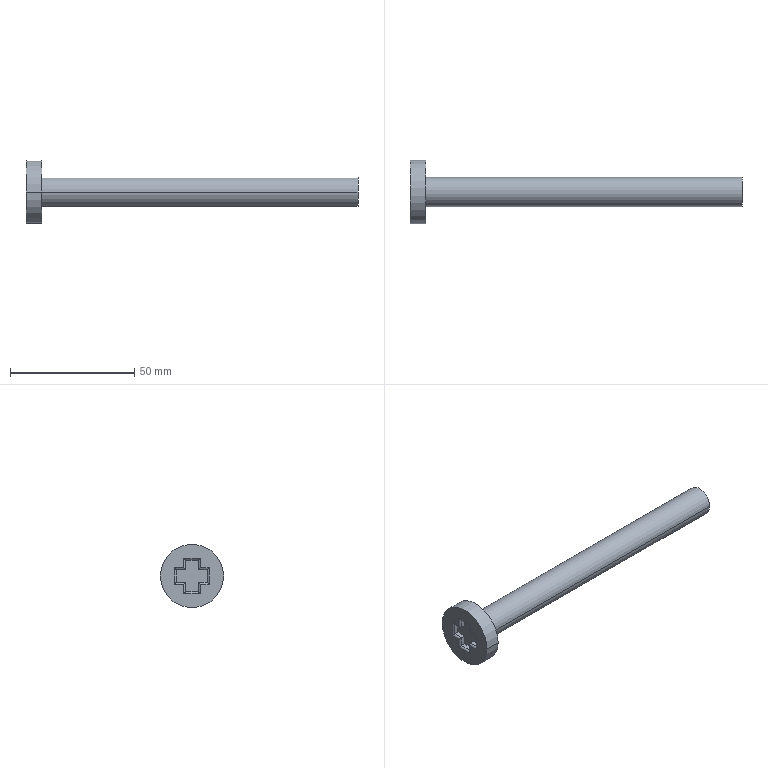Part | SolidWorks | features Fillet 1, ICE 1, Revolution 1 | 1 solid | 32 faces | box 133.35 x 25.4 x 25.4 mm | volume 16568 mm3 | cylinder 16 | plane 16 | commonest cylinder face diameters 1.626 x12 11.684 x2 25.4 x2
STEP:
#1=CARTESIAN_POINT('',(-0.25,0.5,0.));
#2=VERTEX_POINT('',#1);
#3=CARTESIAN_POINT('',(-0.25,-0.5,0.));
#4=VERTEX_POINT('',#3);
#5=CARTESIAN_POINT('',(-0.25,0.,0.));
#6=DIRECTION('',(1.,0.,0.));
#7=DIRECTION('',(0.,1.,0.));
#8=AXIS2_PLACEMENT_3D('',#5,#6,#7);
#9=CIRCLE('',#8,0.5);
#10=EDGE_CURVE('',#2,#4,#9,.T.);
#11=ORIENTED_EDGE('',*,*,#10,.T.);
#12=CARTESIAN_POINT('',(0.,-0.5,0.));
#13=VERTEX_POINT('',#12);
#14=CARTESIAN_POINT('',(5.,-0.5,0.));
#15=DIRECTION('',(1.,0.,0.));
#16=VECTOR('',#15,39.37);
#17=LINE('',#14,#16);
#18=EDGE_CURVE('',#4,#13,#17,.T.);
#19=ORIENTED_EDGE('',*,*,#18,.T.);
#20=CARTESIAN_POINT('',(0.,0.5,0.));
#21=VERTEX_POINT('',#20);
#22=CARTESIAN_POINT('',(0.,0.,0.));
#23=DIRECTION('',(1.,0.,0.));
#24=DIRECTION('',(0.,1.,0.));
#25=AXIS2_PLACEMENT_3D('',#22,#23,#24);
#26=CIRCLE('',#25,0.5);
#27=EDGE_CURVE('',#21,#13,#26,.T.);
#28=ORIENTED_EDGE('',*,*,#27,.F.);
#29=CARTESIAN_POINT('',(5.,0.5,0.));
#30=DIRECTION('',(1.,0.,0.));
#31=VECTOR('',#30,39.37);
#32=LINE('',#29,#31);
#33=EDGE_CURVE('',#2,#21,#32,.T.);
#34=ORIENTED_EDGE('',*,*,#33,.F.);
#35=EDGE_LOOP('',(#11,#19,#28,#34));
#36=FACE_OUTER_BOUND('',#35,.T.);
#37=CARTESIAN_POINT('',(5.,0.,0.));
#38=DIRECTION('',(1.,0.,0.));
#39=DIRECTION('',(0.,1.,0.));
#40=AXIS2_PLACEMENT_3D('',#37,#38,#39);
#41=CYLINDRICAL_SURFACE('',#40,0.5);
#42=ADVANCED_FACE('',(#36),#41,.T.);
#43=CARTESIAN_POINT('',(0.,0.23,0.));
#44=VERTEX_POINT('',#43);
#45=CARTESIAN_POINT('',(0.,-0.23,0.));
#46=VERTEX_POINT('',#45);
#47=CARTESIAN_POINT('',(0.,0.,0.));
#48=DIRECTION('',(1.,0.,0.));
#49=DIRECTION('',(0.,1.,0.));
#50=AXIS2_PLACEMENT_3D('',#47,#48,#49);
#51=CIRCLE('',#50,0.23);
#52=EDGE_CURVE('',#44,#46,#51,.T.);
#53=ORIENTED_EDGE('',*,*,#52,.T.);
#54=CARTESIAN_POINT('',(5.,-0.23,0.));
#55=VERTEX_POINT('',#54);
#56=CARTESIAN_POINT('',(5.,-0.23,0.));
#57=DIRECTION('',(1.,0.,0.));
#58=VECTOR('',#57,39.37);
#59=LINE('',#56,#58);
#60=EDGE_CURVE('',#46,#55,#59,.T.);
#61=ORIENTED_EDGE('',*,*,#60,.T.);
#62=CARTESIAN_POINT('',(5.,0.23,0.));
#63=VERTEX_POINT('',#62);
#64=CARTESIAN_POINT('',(5.,0.,0.));
#65=DIRECTION('',(1.,0.,0.));
#66=DIRECTION('',(0.,1.,0.));
#67=AXIS2_PLACEMENT_3D('',#64,#65,#66);
#68=CIRCLE('',#67,0.23);
#69=EDGE_CURVE('',#63,#55,#68,.T.);
#70=ORIENTED_EDGE('',*,*,#69,.F.);
#71=CARTESIAN_POINT('',(5.,0.23,0.));
#72=DIRECTION('',(1.,0.,0.));
#73=VECTOR('',#72,39.37);
#74=LINE('',#71,#73);
#75=EDGE_CURVE('',#44,#63,#74,.T.);
#76=ORIENTED_EDGE('',*,*,#75,.F.);
#77=EDGE_LOOP('',(#53,#61,#70,#76));
#78=FACE_OUTER_BOUND('',#77,.T.);
#79=CARTESIAN_POINT('',(5.,0.,0.));
#80=DIRECTION('',(1.,0.,0.));
#81=DIRECTION('',(0.,1.,0.));
#82=AXIS2_PLACEMENT_3D('',#79,#80,#81);
#83=CYLINDRICAL_SURFACE('',#82,0.23);
#84=ADVANCED_FACE('',(#78),#83,.T.);
#85=ORIENTED_EDGE('',*,*,#69,.T.);
#86=CARTESIAN_POINT('',(5.,0.,0.));
#87=DIRECTION('',(1.,0.,0.));
#88=DIRECTION('',(0.,1.,0.));
#89=AXIS2_PLACEMENT_3D('',#86,#87,#88);
#90=CIRCLE('',#89,0.23);
#91=EDGE_CURVE('',#55,#63,#90,.T.);
#92=ORIENTED_EDGE('',*,*,#91,.T.);
#93=EDGE_LOOP('',(#85,#92));
#94=FACE_OUTER_BOUND('',#93,.T.);
#95=CARTESIAN_POINT('',(5.,0.23,0.));
#96=DIRECTION('',(1.,0.,0.));
#97=DIRECTION('',(0.,1.,0.));
#98=AXIS2_PLACEMENT_3D('',#95,#96,#97);
#99=PLANE('',#98);
#100=ADVANCED_FACE('',(#94),#99,.T.);
#101=ORIENTED_EDGE('',*,*,#60,.F.);
#102=CARTESIAN_POINT('',(0.,0.,0.));
#103=DIRECTION('',(1.,0.,0.));
#104=DIRECTION('',(0.,1.,0.));
#105=AXIS2_PLACEMENT_3D('',#102,#103,#104);
#106=CIRCLE('',#105,0.23);
#107=EDGE_CURVE('',#46,#44,#106,.T.);
#108=ORIENTED_EDGE('',*,*,#107,.T.);
#109=ORIENTED_EDGE('',*,*,#75,.T.);
#110=ORIENTED_EDGE('',*,*,#91,.F.);
#111=EDGE_LOOP('',(#101,#108,#109,#110));
#112=FACE_OUTER_BOUND('',#111,.T.);
#113=CARTESIAN_POINT('',(5.,0.,0.));
#114=DIRECTION('',(1.,0.,0.));
#115=DIRECTION('',(0.,1.,0.));
#116=AXIS2_PLACEMENT_3D('',#113,#114,#115);
#117=CYLINDRICAL_SURFACE('',#116,0.23);
#118=ADVANCED_FACE('',(#112),#117,.T.);
#119=ORIENTED_EDGE('',*,*,#27,.T.);
#120=CARTESIAN_POINT('',(0.,0.,0.));
#121=DIRECTION('',(1.,0.,0.));
#122=DIRECTION('',(0.,1.,0.));
#123=AXIS2_PLACEMENT_3D('',#120,#121,#122);
#124=CIRCLE('',#123,0.5);
#125=EDGE_CURVE('',#13,#21,#124,.T.);
#126=ORIENTED_EDGE('',*,*,#125,.T.);
#127=EDGE_LOOP('',(#119,#126));
#128=FACE_OUTER_BOUND('',#127,.T.);
#129=ORIENTED_EDGE('',*,*,#52,.F.);
#130=ORIENTED_EDGE('',*,*,#107,.F.);
#131=EDGE_LOOP('',(#129,#130));
#132=FACE_BOUND('',#131,.T.);
#133=CARTESIAN_POINT('',(0.,0.23,0.));
#134=DIRECTION('',(1.,0.,0.));
#135=DIRECTION('',(0.,1.,0.));
#136=AXIS2_PLACEMENT_3D('',#133,#134,#135);
#137=PLANE('',#136);
#138=ADVANCED_FACE('',(#128,#132),#137,.T.);
#139=ORIENTED_EDGE('',*,*,#18,.F.);
#140=CARTESIAN_POINT('',(-0.25,0.,0.));
#141=DIRECTION('',(1.,0.,0.));
#142=DIRECTION('',(0.,1.,0.));
#143=AXIS2_PLACEMENT_3D('',#140,#141,#142);
#144=CIRCLE('',#143,0.5);
#145=EDGE_CURVE('',#4,#2,#144,.T.);
#146=ORIENTED_EDGE('',*,*,#145,.T.);
#147=ORIENTED_EDGE('',*,*,#33,.T.);
#148=ORIENTED_EDGE('',*,*,#125,.F.);
#149=EDGE_LOOP('',(#139,#146,#147,#148));
#150=FACE_OUTER_BOUND('',#149,.T.);
#151=CARTESIAN_POINT('',(5.,0.,0.));
#152=DIRECTION('',(1.,0.,0.));
#153=DIRECTION('',(0.,1.,0.));
#154=AXIS2_PLACEMENT_3D('',#151,#152,#153);
#155=CYLINDRICAL_SURFACE('',#154,0.5);
#156=ADVANCED_FACE('',(#150),#155,.T.);
#157=CARTESIAN_POINT('',(-0.25,-0.132,0.132));
#158=VERTEX_POINT('',#157);
#159=CARTESIAN_POINT('',(-0.25,-0.273,0.132));
#160=VERTEX_POINT('',#159);
#161=CARTESIAN_POINT('',(-0.25,-0.241,0.132));
#162=DIRECTION('',(0.,-1.,0.));
#163=VECTOR('',#162,39.37);
#164=LINE('',#161,#163);
#165=EDGE_CURVE('',#158,#160,#164,.T.);
#166=ORIENTED_EDGE('',*,*,#165,.T.);
#167=CARTESIAN_POINT('',(-0.25,-0.273,-0.132));
#168=VERTEX_POINT('',#167);
#169=CARTESIAN_POINT('',(-0.25,-0.273,-0.1));
#170=DIRECTION('',(0.,0.,-1.));
#171=VECTOR('',#170,39.37);
#172=LINE('',#169,#171);
#173=EDGE_CURVE('',#160,#168,#172,.T.);
#174=ORIENTED_EDGE('',*,*,#173,.T.);
#175=CARTESIAN_POINT('',(-0.25,-0.132,-0.132));
#176=VERTEX_POINT('',#175);
#177=CARTESIAN_POINT('',(-0.25,-0.1,-0.132));
#178=DIRECTION('',(0.,1.,0.));
#179=VECTOR('',#178,39.37);
#180=LINE('',#177,#179);
#181=EDGE_CURVE('',#168,#176,#180,.T.);
#182=ORIENTED_EDGE('',*,*,#181,.T.);
#183=CARTESIAN_POINT('',(-0.25,-0.132,-0.282));
#184=VERTEX_POINT('',#183);
#185=CARTESIAN_POINT('',(-0.25,-0.132,-0.25));
#186=DIRECTION('',(0.,0.,-1.));
#187=VECTOR('',#186,39.37);
#188=LINE('',#185,#187);
#189=EDGE_CURVE('',#176,#184,#188,.T.);
#190=ORIENTED_EDGE('',*,*,#189,.T.);
#191=CARTESIAN_POINT('',(-0.25,0.132,-0.282));
#192=VERTEX_POINT('',#191);
#193=CARTESIAN_POINT('',(-0.25,0.1,-0.282));
#194=DIRECTION('',(0.,1.,0.));
#195=VECTOR('',#194,39.37);
#196=LINE('',#193,#195);
#197=EDGE_CURVE('',#184,#192,#196,.T.);
#198=ORIENTED_EDGE('',*,*,#197,.T.);
#199=CARTESIAN_POINT('',(-0.25,0.132,-0.132));
#200=VERTEX_POINT('',#199);
#201=CARTESIAN_POINT('',(-0.25,0.132,-0.1));
#202=DIRECTION('',(0.,0.,1.));
#203=VECTOR('',#202,39.37);
#204=LINE('',#201,#203);
#205=EDGE_CURVE('',#192,#200,#204,.T.);
#206=ORIENTED_EDGE('',*,*,#205,.T.);
#207=CARTESIAN_POINT('',(-0.25,0.282,-0.132));
#208=VERTEX_POINT('',#207);
#209=CARTESIAN_POINT('',(-0.25,0.25,-0.132));
#210=DIRECTION('',(0.,1.,0.));
#211=VECTOR('',#210,39.37);
#212=LINE('',#209,#211);
#213=EDGE_CURVE('',#200,#208,#212,.T.);
#214=ORIENTED_EDGE('',*,*,#213,.T.);
#215=CARTESIAN_POINT('',(-0.25,0.282,0.132));
#216=VERTEX_POINT('',#215);
#217=CARTESIAN_POINT('',(-0.25,0.282,0.1));
#218=DIRECTION('',(0.,0.,1.));
#219=VECTOR('',#218,39.37);
#220=LINE('',#217,#219);
#221=EDGE_CURVE('',#208,#216,#220,.T.);
#222=ORIENTED_EDGE('',*,*,#221,.T.);
#223=CARTESIAN_POINT('',(-0.25,0.132,0.132));
#224=VERTEX_POINT('',#223);
#225=CARTESIAN_POINT('',(-0.25,0.1,0.132));
#226=DIRECTION('',(0.,-1.,0.));
#227=VECTOR('',#226,39.37);
#228=LINE('',#225,#227);
#229=EDGE_CURVE('',#216,#224,#228,.T.);
#230=ORIENTED_EDGE('',*,*,#229,.T.);
#231=CARTESIAN_POINT('',(-0.25,0.132,0.282));
#232=VERTEX_POINT('',#231);
#233=CARTESIAN_POINT('',(-0.25,0.132,0.25));
#234=DIRECTION('',(0.,0.,1.));
#235=VECTOR('',#234,39.37);
#236=LINE('',#233,#235);
#237=EDGE_CURVE('',#224,#232,#236,.T.);
#238=ORIENTED_EDGE('',*,*,#237,.T.);
#239=CARTESIAN_POINT('',(-0.25,-0.132,0.282));
#240=VERTEX_POINT('',#239);
#241=CARTESIAN_POINT('',(-0.25,-0.1,0.282));
#242=DIRECTION('',(0.,-1.,0.));
#243=VECTOR('',#242,39.37);
#244=LINE('',#241,#243);
#245=EDGE_CURVE('',#232,#240,#244,.T.);
#246=ORIENTED_EDGE('',*,*,#245,.T.);
#247=CARTESIAN_POINT('',(-0.25,-0.132,0.1));
#248=DIRECTION('',(0.,0.,-1.));
#249=VECTOR('',#248,39.37);
#250=LINE('',#247,#249);
#251=EDGE_CURVE('',#240,#158,#250,.T.);
#252=ORIENTED_EDGE('',*,*,#251,.T.);
#253=EDGE_LOOP('',(#166,#174,#182,#190,#198,#206,#214,#222,#230,#238,#246,#252));
#254=FACE_BOUND('',#253,.T.);
#255=ORIENTED_EDGE('',*,*,#10,.F.);
#256=ORIENTED_EDGE('',*,*,#145,.F.);
#257=EDGE_LOOP('',(#255,#256));
#258=FACE_OUTER_BOUND('',#257,.T.);
#259=CARTESIAN_POINT('',(-0.25,0.5,0.));
#260=DIRECTION('',(-1.,0.,0.));
#261=DIRECTION('',(0.,-1.,0.));
#262=AXIS2_PLACEMENT_3D('',#259,#260,#261);
#263=PLANE('',#262);
#264=ADVANCED_FACE('',(#254,#258),#263,.T.);
#265=CARTESIAN_POINT('',(-0.15,0.25,0.1));
#266=VERTEX_POINT('',#265);
#267=CARTESIAN_POINT('',(-0.218,0.25,0.1));
#268=VERTEX_POINT('',#267);
#269=CARTESIAN_POINT('',(-0.15,0.25,0.1));
#270=DIRECTION('',(-1.,0.,0.));
#271=VECTOR('',#270,39.37);
#272=LINE('',#269,#271);
#273=EDGE_CURVE('',#266,#268,#272,.T.);
#274=ORIENTED_EDGE('',*,*,#273,.T.);
#275=CARTESIAN_POINT('',(-0.218,0.25,-0.1));
#276=VERTEX_POINT('',#275);
#277=CARTESIAN_POINT('',(-0.218,0.25,-0.1));
#278=DIRECTION('',(0.,0.,-1.));
#279=VECTOR('',#278,39.37);
#280=LINE('',#277,#279);
#281=EDGE_CURVE('',#268,#276,#280,.T.);
#282=ORIENTED_EDGE('',*,*,#281,.T.);
#283=CARTESIAN_POINT('',(-0.15,0.25,-0.1));
#284=VERTEX_POINT('',#283);
#285=CARTESIAN_POINT('',(-0.15,0.25,-0.1));
#286=DIRECTION('',(-1.,0.,0.));
#287=VECTOR('',#286,39.37);
#288=LINE('',#285,#287);
#289=EDGE_CURVE('',#284,#276,#288,.T.);
#290=ORIENTED_EDGE('',*,*,#289,.F.);
#291=CARTESIAN_POINT('',(-0.15,0.25,-0.1));
#292=DIRECTION('',(0.,0.,-1.));
#293=VECTOR('',#292,39.37);
#294=LINE('',#291,#293);
#295=EDGE_CURVE('',#266,#284,#294,.T.);
#296=ORIENTED_EDGE('',*,*,#295,.F.);
#297=EDGE_LOOP('',(#274,#282,#290,#296));
#298=FACE_OUTER_BOUND('',#297,.T.);
#299=CARTESIAN_POINT('',(-0.15,0.25,-0.1));
#300=DIRECTION('',(0.,1.,0.));
#301=DIRECTION('',(-1.,0.,0.));
#302=AXIS2_PLACEMENT_3D('',#299,#300,#301);
#303=PLANE('',#302);
#304=ADVANCED_FACE('',(#298),#303,.F.);
#305=CARTESIAN_POINT('',(-0.15,0.1,0.1));
#306=VERTEX_POINT('',#305);
#307=CARTESIAN_POINT('',(-0.218,0.1,0.1));
#308=VERTEX_POINT('',#307);
#309=CARTESIAN_POINT('',(-0.15,0.1,0.1));
#310=DIRECTION('',(-1.,0.,0.));
#311=VECTOR('',#310,39.37);
#312=LINE('',#309,#311);
#313=EDGE_CURVE('',#306,#308,#312,.T.);
#314=ORIENTED_EDGE('',*,*,#313,.T.);
#315=CARTESIAN_POINT('',(-0.218,0.25,0.1));
#316=DIRECTION('',(0.,1.,0.));
#317=VECTOR('',#316,39.37);
#318=LINE('',#315,#317);
#319=EDGE_CURVE('',#308,#268,#318,.T.);
#320=ORIENTED_EDGE('',*,*,#319,.T.);
#321=ORIENTED_EDGE('',*,*,#273,.F.);
#322=CARTESIAN_POINT('',(-0.15,0.25,0.1));
#323=DIRECTION('',(0.,1.,0.));
#324=VECTOR('',#323,39.37);
#325=LINE('',#322,#324);
#326=EDGE_CURVE('',#306,#266,#325,.T.);
#327=ORIENTED_EDGE('',*,*,#326,.F.);
#328=EDGE_LOOP('',(#314,#320,#321,#327));
#329=FACE_OUTER_BOUND('',#328,.T.);
#330=CARTESIAN_POINT('',(-0.15,0.25,0.1));
#331=DIRECTION('',(0.,0.,1.));
#332=DIRECTION('',(0.,-1.,0.));
#333=AXIS2_PLACEMENT_3D('',#330,#331,#332);
#334=PLANE('',#333);
#335=ADVANCED_FACE('',(#329),#334,.F.);
#336=CARTESIAN_POINT('',(-0.15,0.1,0.25));
#337=VERTEX_POINT('',#336);
#338=CARTESIAN_POINT('',(-0.218,0.1,0.25));
#339=VERTEX_POINT('',#338);
#340=CARTESIAN_POINT('',(-0.15,0.1,0.25));
#341=DIRECTION('',(-1.,0.,0.));
#342=VECTOR('',#341,39.37);
#343=LINE('',#340,#342);
#344=EDGE_CURVE('',#337,#339,#343,.T.);
#345=ORIENTED_EDGE('',*,*,#344,.T.);
#346=CARTESIAN_POINT('',(-0.218,0.1,0.1));
#347=DIRECTION('',(0.,0.,-1.));
#348=VECTOR('',#347,39.37);
#349=LINE('',#346,#348);
#350=EDGE_CURVE('',#339,#308,#349,.T.);
#351=ORIENTED_EDGE('',*,*,#350,.T.);
#352=ORIENTED_EDGE('',*,*,#313,.F.);
#353=CARTESIAN_POINT('',(-0.15,0.1,0.1));
#354=DIRECTION('',(0.,0.,-1.));
#355=VECTOR('',#354,39.37);
#356=LINE('',#353,#355);
#357=EDGE_CURVE('',#337,#306,#356,.T.);
#358=ORIENTED_EDGE('',*,*,#357,.F.);
#359=EDGE_LOOP('',(#345,#351,#352,#358));
#360=FACE_OUTER_BOUND('',#359,.T.);
#361=CARTESIAN_POINT('',(-0.15,0.1,0.1));
#362=DIRECTION('',(0.,1.,0.));
#363=DIRECTION('',(-1.,0.,0.));
#364=AXIS2_PLACEMENT_3D('',#361,#362,#363);
#365=PLANE('',#364);
#366=ADVANCED_FACE('',(#360),#365,.F.);
#367=CARTESIAN_POINT('',(-0.15,-0.1,0.25));
#368=VERTEX_POINT('',#367);
#369=CARTESIAN_POINT('',(-0.218,-0.1,0.25));
#370=VERTEX_POINT('',#369);
#371=CARTESIAN_POINT('',(-0.15,-0.1,0.25));
#372=DIRECTION('',(-1.,0.,0.));
#373=VECTOR('',#372,39.37);
#374=LINE('',#371,#373);
#375=EDGE_CURVE('',#368,#370,#374,.T.);
#376=ORIENTED_EDGE('',*,*,#375,.T.);
#377=CARTESIAN_POINT('',(-0.218,0.1,0.25));
#378=DIRECTION('',(0.,1.,0.));
#379=VECTOR('',#378,39.37);
#380=LINE('',#377,#379);
#381=EDGE_CURVE('',#370,#339,#380,.T.);
#382=ORIENTED_EDGE('',*,*,#381,.T.);
#383=ORIENTED_EDGE('',*,*,#344,.F.);
#384=CARTESIAN_POINT('',(-0.15,0.1,0.25));
#385=DIRECTION('',(0.,1.,0.));
#386=VECTOR('',#385,39.37);
#387=LINE('',#384,#386);
#388=EDGE_CURVE('',#368,#337,#387,.T.);
#389=ORIENTED_EDGE('',*,*,#388,.F.);
#390=EDGE_LOOP('',(#376,#382,#383,#389));
#391=FACE_OUTER_BOUND('',#390,.T.);
#392=CARTESIAN_POINT('',(-0.15,0.1,0.25));
#393=DIRECTION('',(0.,0.,1.));
#394=DIRECTION('',(0.,-1.,0.));
#395=AXIS2_PLACEMENT_3D('',#392,#393,#394);
#396=PLANE('',#395);
#397=ADVANCED_FACE('',(#391),#396,.F.);
#398=CARTESIAN_POINT('',(-0.15,-0.1,0.1));
#399=VERTEX_POINT('',#398);
#400=CARTESIAN_POINT('',(-0.218,-0.1,0.1));
#401=VERTEX_POINT('',#400);
#402=CARTESIAN_POINT('',(-0.15,-0.1,0.1));
#403=DIRECTION('',(-1.,0.,0.));
#404=VECTOR('',#403,39.37);
#405=LINE('',#402,#404);
#406=EDGE_CURVE('',#399,#401,#405,.T.);
#407=ORIENTED_EDGE('',*,*,#406,.T.);
#408=CARTESIAN_POINT('',(-0.218,-0.1,0.25));
#409=DIRECTION('',(0.,0.,1.));
#410=VECTOR('',#409,39.37);
#411=LINE('',#408,#410);
#412=EDGE_CURVE('',#401,#370,#411,.T.);
#413=ORIENTED_EDGE('',*,*,#412,.T.);
#414=ORIENTED_EDGE('',*,*,#375,.F.);
#415=CARTESIAN_POINT('',(-0.15,-0.1,0.25));
#416=DIRECTION('',(0.,0.,1.));
#417=VECTOR('',#416,39.37);
#418=LINE('',#415,#417);
#419=EDGE_CURVE('',#399,#368,#418,.T.);
#420=ORIENTED_EDGE('',*,*,#419,.F.);
#421=EDGE_LOOP('',(#407,#413,#414,#420));
#422=FACE_OUTER_BOUND('',#421,.T.);
#423=CARTESIAN_POINT('',(-0.15,-0.1,0.25));
#424=DIRECTION('',(0.,-1.,0.));
#425=DIRECTION('',(0.,0.,-1.));
#426=AXIS2_PLACEMENT_3D('',#423,#424,#425);
#427=PLANE('',#426);
#428=ADVANCED_FACE('',(#422),#427,.F.);
#429=CARTESIAN_POINT('',(-0.15,-0.241,0.1));
#430=VERTEX_POINT('',#429);
#431=CARTESIAN_POINT('',(-0.218,-0.241,0.1));
#432=VERTEX_POINT('',#431);
#433=CARTESIAN_POINT('',(-0.15,-0.241,0.1));
#434=DIRECTION('',(-1.,0.,0.));
#435=VECTOR('',#434,39.37);
#436=LINE('',#433,#435);
#437=EDGE_CURVE('',#430,#432,#436,.T.);
#438=ORIENTED_EDGE('',*,*,#437,.T.);
#439=CARTESIAN_POINT('',(-0.218,-0.1,0.1));
#440=DIRECTION('',(0.,1.,0.));
#441=VECTOR('',#440,39.37);
#442=LINE('',#439,#441);
#443=EDGE_CURVE('',#432,#401,#442,.T.);
#444=ORIENTED_EDGE('',*,*,#443,.T.);
#445=ORIENTED_EDGE('',*,*,#406,.F.);
#446=CARTESIAN_POINT('',(-0.15,-0.1,0.1));
#447=DIRECTION('',(0.,1.,0.));
#448=VECTOR('',#447,39.37);
#449=LINE('',#446,#448);
#450=EDGE_CURVE('',#430,#399,#449,.T.);
#451=ORIENTED_EDGE('',*,*,#450,.F.);
#452=EDGE_LOOP('',(#438,#444,#445,#451));
#453=FACE_OUTER_BOUND('',#452,.T.);
#454=CARTESIAN_POINT('',(-0.15,-0.1,0.1));
#455=DIRECTION('',(0.,0.,1.));
#456=DIRECTION('',(0.,-1.,0.));
#457=AXIS2_PLACEMENT_3D('',#454,#455,#456);
#458=PLANE('',#457);
#459=ADVANCED_FACE('',(#453),#458,.F.);
#460=CARTESIAN_POINT('',(-0.15,-0.241,-0.1));
#461=VERTEX_POINT('',#460);
#462=CARTESIAN_POINT('',(-0.218,-0.241,-0.1));
#463=VERTEX_POINT('',#462);
#464=CARTESIAN_POINT('',(-0.15,-0.241,-0.1));
#465=DIRECTION('',(-1.,0.,0.));
#466=VECTOR('',#465,39.37);
#467=LINE('',#464,#466);
#468=EDGE_CURVE('',#461,#463,#467,.T.);
#469=ORIENTED_EDGE('',*,*,#468,.T.);
#470=CARTESIAN_POINT('',(-0.218,-0.241,0.1));
#471=DIRECTION('',(0.,0.,1.));
#472=VECTOR('',#471,39.37);
#473=LINE('',#470,#472);
#474=EDGE_CURVE('',#463,#432,#473,.T.);
#475=ORIENTED_EDGE('',*,*,#474,.T.);
#476=ORIENTED_EDGE('',*,*,#437,.F.);
#477=CARTESIAN_POINT('',(-0.15,-0.241,-0.1));
#478=DIRECTION('',(0.,0.,1.));
#479=VECTOR('',#478,39.37);
#480=LINE('',#477,#479);
#481=EDGE_CURVE('',#461,#430,#480,.T.);
#482=ORIENTED_EDGE('',*,*,#481,.F.);
#483=EDGE_LOOP('',(#469,#475,#476,#482));
#484=FACE_OUTER_BOUND('',#483,.T.);
#485=CARTESIAN_POINT('',(-0.15,-0.241,-0.1));
#486=DIRECTION('',(0.,-1.,0.));
#487=DIRECTION('',(1.,0.,0.));
#488=AXIS2_PLACEMENT_3D('',#485,#486,#487);
#489=PLANE('',#488);
#490=ADVANCED_FACE('',(#484),#489,.F.);
#491=CARTESIAN_POINT('',(-0.15,-0.1,-0.1));
#492=VERTEX_POINT('',#491);
#493=CARTESIAN_POINT('',(-0.218,-0.1,-0.1));
#494=VERTEX_POINT('',#493);
#495=CARTESIAN_POINT('',(-0.15,-0.1,-0.1));
#496=DIRECTION('',(-1.,0.,0.));
#497=VECTOR('',#496,39.37);
#498=LINE('',#495,#497);
#499=EDGE_CURVE('',#492,#494,#498,.T.);
#500=ORIENTED_EDGE('',*,*,#499,.T.);
#501=CARTESIAN_POINT('',(-0.218,-0.241,-0.1));
#502=DIRECTION('',(0.,-1.,0.));
#503=VECTOR('',#502,39.37);
#504=LINE('',#501,#503);
#505=EDGE_CURVE('',#494,#463,#504,.T.);
#506=ORIENTED_EDGE('',*,*,#505,.T.);
#507=ORIENTED_EDGE('',*,*,#468,.F.);
#508=CARTESIAN_POINT('',(-0.15,-0.1,-0.1));
#509=DIRECTION('',(0.,-1.,0.));
#510=VECTOR('',#509,39.37);
#511=LINE('',#508,#510);
#512=EDGE_CURVE('',#492,#461,#511,.T.);
#513=ORIENTED_EDGE('',*,*,#512,.F.);
#514=EDGE_LOOP('',(#500,#506,#507,#513));
#515=FACE_OUTER_BOUND('',#514,.T.);
#516=CARTESIAN_POINT('',(-0.15,-0.1,-0.1));
#517=DIRECTION('',(0.,0.,-1.));
#518=DIRECTION('',(0.,1.,0.));
#519=AXIS2_PLACEMENT_3D('',#516,#517,#518);
#520=PLANE('',#519);
#521=ADVANCED_FACE('',(#515),#520,.F.);
#522=CARTESIAN_POINT('',(-0.15,-0.1,-0.25));
#523=VERTEX_POINT('',#522);
#524=CARTESIAN_POINT('',(-0.218,-0.1,-0.25));
#525=VERTEX_POINT('',#524);
#526=CARTESIAN_POINT('',(-0.15,-0.1,-0.25));
#527=DIRECTION('',(-1.,0.,0.));
#528=VECTOR('',#527,39.37);
#529=LINE('',#526,#528);
#530=EDGE_CURVE('',#523,#525,#529,.T.);
#531=ORIENTED_EDGE('',*,*,#530,.T.);
#532=CARTESIAN_POINT('',(-0.218,-0.1,-0.1));
#533=DIRECTION('',(0.,0.,1.));
#534=VECTOR('',#533,39.37);
#535=LINE('',#532,#534);
#536=EDGE_CURVE('',#525,#494,#535,.T.);
#537=ORIENTED_EDGE('',*,*,#536,.T.);
#538=ORIENTED_EDGE('',*,*,#499,.F.);
#539=CARTESIAN_POINT('',(-0.15,-0.1,-0.25));
#540=DIRECTION('',(0.,0.,1.));
#541=VECTOR('',#540,39.37);
#542=LINE('',#539,#541);
#543=EDGE_CURVE('',#523,#492,#542,.T.);
#544=ORIENTED_EDGE('',*,*,#543,.F.);
#545=EDGE_LOOP('',(#531,#537,#538,#544));
#546=FACE_OUTER_BOUND('',#545,.T.);
#547=CARTESIAN_POINT('',(-0.15,-0.1,-0.25));
#548=DIRECTION('',(0.,-1.,0.));
#549=DIRECTION('',(0.,0.,-1.));
#550=AXIS2_PLACEMENT_3D('',#547,#548,#549);
#551=PLANE('',#550);
#552=ADVANCED_FACE('',(#546),#551,.F.);
#553=CARTESIAN_POINT('',(-0.15,0.1,-0.25));
#554=VERTEX_POINT('',#553);
#555=CARTESIAN_POINT('',(-0.218,0.1,-0.25));
#556=VERTEX_POINT('',#555);
#557=CARTESIAN_POINT('',(-0.15,0.1,-0.25));
#558=DIRECTION('',(-1.,0.,0.));
#559=VECTOR('',#558,39.37);
#560=LINE('',#557,#559);
#561=EDGE_CURVE('',#554,#556,#560,.T.);
#562=ORIENTED_EDGE('',*,*,#561,.T.);
#563=CARTESIAN_POINT('',(-0.218,-0.1,-0.25));
#564=DIRECTION('',(0.,-1.,0.));
#565=VECTOR('',#564,39.37);
#566=LINE('',#563,#565);
#567=EDGE_CURVE('',#556,#525,#566,.T.);
#568=ORIENTED_EDGE('',*,*,#567,.T.);
#569=ORIENTED_EDGE('',*,*,#530,.F.);
#570=CARTESIAN_POINT('',(-0.15,0.1,-0.25));
#571=DIRECTION('',(0.,-1.,0.));
#572=VECTOR('',#571,39.37);
#573=LINE('',#570,#572);
#574=EDGE_CURVE('',#554,#523,#573,.T.);
#575=ORIENTED_EDGE('',*,*,#574,.F.);
#576=EDGE_LOOP('',(#562,#568,#569,#575));
#577=FACE_OUTER_BOUND('',#576,.T.);
#578=CARTESIAN_POINT('',(-0.15,0.1,-0.25));
#579=DIRECTION('',(0.,0.,-1.));
#580=DIRECTION('',(0.,1.,0.));
#581=AXIS2_PLACEMENT_3D('',#578,#579,#580);
#582=PLANE('',#581);
#583=ADVANCED_FACE('',(#577),#582,.F.);
#584=CARTESIAN_POINT('',(-0.15,0.1,-0.1));
#585=VERTEX_POINT('',#584);
#586=CARTESIAN_POINT('',(-0.218,0.1,-0.1));
#587=VERTEX_POINT('',#586);
#588=CARTESIAN_POINT('',(-0.15,0.1,-0.1));
#589=DIRECTION('',(-1.,0.,0.));
#590=VECTOR('',#589,39.37);
#591=LINE('',#588,#590);
#592=EDGE_CURVE('',#585,#587,#591,.T.);
#593=ORIENTED_EDGE('',*,*,#592,.T.);
#594=CARTESIAN_POINT('',(-0.218,0.1,-0.25));
#595=DIRECTION('',(0.,0.,-1.));
#596=VECTOR('',#595,39.37);
#597=LINE('',#594,#596);
#598=EDGE_CURVE('',#587,#556,#597,.T.);
#599=ORIENTED_EDGE('',*,*,#598,.T.);
#600=ORIENTED_EDGE('',*,*,#561,.F.);
#601=CARTESIAN_POINT('',(-0.15,0.1,-0.1));
#602=DIRECTION('',(0.,0.,-1.));
#603=VECTOR('',#602,39.37);
#604=LINE('',#601,#603);
#605=EDGE_CURVE('',#585,#554,#604,.T.);
#606=ORIENTED_EDGE('',*,*,#605,.F.);
#607=EDGE_LOOP('',(#593,#599,#600,#606));
#608=FACE_OUTER_BOUND('',#607,.T.);
#609=CARTESIAN_POINT('',(-0.15,0.1,-0.1));
#610=DIRECTION('',(0.,1.,0.));
#611=DIRECTION('',(-1.,0.,0.));
#612=AXIS2_PLACEMENT_3D('',#609,#610,#611);
#613=PLANE('',#612);
#614=ADVANCED_FACE('',(#608),#613,.F.);
#615=ORIENTED_EDGE('',*,*,#289,.T.);
#616=CARTESIAN_POINT('',(-0.218,0.1,-0.1));
#617=DIRECTION('',(0.,-1.,0.));
#618=VECTOR('',#617,39.37);
#619=LINE('',#616,#618);
#620=EDGE_CURVE('',#276,#587,#619,.T.);
#621=ORIENTED_EDGE('',*,*,#620,.T.);
#622=ORIENTED_EDGE('',*,*,#592,.F.);
#623=CARTESIAN_POINT('',(-0.15,0.25,-0.1));
#624=DIRECTION('',(0.,-1.,0.));
#625=VECTOR('',#624,39.37);
#626=LINE('',#623,#625);
#627=EDGE_CURVE('',#284,#585,#626,.T.);
#628=ORIENTED_EDGE('',*,*,#627,.F.);
#629=EDGE_LOOP('',(#615,#621,#622,#628));
#630=FACE_OUTER_BOUND('',#629,.T.);
#631=CARTESIAN_POINT('',(-0.15,0.25,-0.1));
#632=DIRECTION('',(0.,0.,-1.));
#633=DIRECTION('',(0.,1.,0.));
#634=AXIS2_PLACEMENT_3D('',#631,#632,#633);
#635=PLANE('',#634);
#636=ADVANCED_FACE('',(#630),#635,.F.);
#637=ORIENTED_EDGE('',*,*,#295,.T.);
#638=ORIENTED_EDGE('',*,*,#627,.T.);
#639=ORIENTED_EDGE('',*,*,#605,.T.);
#640=ORIENTED_EDGE('',*,*,#574,.T.);
#641=ORIENTED_EDGE('',*,*,#543,.T.);
#642=ORIENTED_EDGE('',*,*,#512,.T.);
#643=ORIENTED_EDGE('',*,*,#481,.T.);
#644=ORIENTED_EDGE('',*,*,#450,.T.);
#645=ORIENTED_EDGE('',*,*,#419,.T.);
#646=ORIENTED_EDGE('',*,*,#388,.T.);
#647=ORIENTED_EDGE('',*,*,#357,.T.);
#648=ORIENTED_EDGE('',*,*,#326,.T.);
#649=EDGE_LOOP('',(#637,#638,#639,#640,#641,#642,#643,#644,#645,#646,#647,#648));
#650=FACE_OUTER_BOUND('',#649,.T.);
#651=CARTESIAN_POINT('',(-0.15,0.,0.));
#652=DIRECTION('',(1.,0.,0.));
#653=DIRECTION('',(0.,0.,-1.));
#654=AXIS2_PLACEMENT_3D('',#651,#652,#653);
#655=PLANE('',#654);
#656=ADVANCED_FACE('',(#650),#655,.F.);
#657=CARTESIAN_POINT('',(-0.25,-0.132,0.282));
#658=CARTESIAN_POINT('',(-0.25,-0.1133,0.2633));
#659=CARTESIAN_POINT('',(-0.2367,-0.1,0.25));
#660=CARTESIAN_POINT('',(-0.218,-0.1,0.25));
#661=(BOUNDED_CURVE()B_SPLINE_CURVE(3,(#657,#658,#659,#660),.UNSPECIFIED.,.F.,.F.)B_SPLINE_CURVE_WITH_KNOTS((4,4),(1.571,3.142),.UNSPECIFIED.)CURVE()GEOMETRIC_REPRESENTATION_ITEM()RATIONAL_B_SPLINE_CURVE((1.,0.8047,0.8047,1.))REPRESENTATION_ITEM(''));
#662=EDGE_CURVE('',#240,#370,#661,.T.);
#663=ORIENTED_EDGE('',*,*,#662,.F.);
#664=ORIENTED_EDGE('',*,*,#245,.F.);
#665=CARTESIAN_POINT('',(-0.218,0.1,0.25));
#666=CARTESIAN_POINT('',(-0.2367,0.1,0.25));
#667=CARTESIAN_POINT('',(-0.25,0.1133,0.2633));
#668=CARTESIAN_POINT('',(-0.25,0.132,0.282));
#669=(BOUNDED_CURVE()B_SPLINE_CURVE(3,(#665,#666,#667,#668),.UNSPECIFIED.,.F.,.T.)B_SPLINE_CURVE_WITH_KNOTS((4,4),(0.,1.571),.UNSPECIFIED.)CURVE()GEOMETRIC_REPRESENTATION_ITEM()RATIONAL_B_SPLINE_CURVE((1.,0.8047,0.8047,1.))REPRESENTATION_ITEM(''));
#670=EDGE_CURVE('',#339,#232,#669,.T.);
#671=ORIENTED_EDGE('',*,*,#670,.F.);
#672=ORIENTED_EDGE('',*,*,#381,.F.);
#673=EDGE_LOOP('',(#663,#664,#671,#672));
#674=FACE_OUTER_BOUND('',#673,.T.);
#675=CARTESIAN_POINT('',(-0.218,0.1,0.282));
#676=DIRECTION('',(0.,-1.,0.));
#677=DIRECTION('',(0.,0.,-1.));
#678=AXIS2_PLACEMENT_3D('',#675,#676,#677);
#679=CYLINDRICAL_SURFACE('',#678,0.032);
#680=ADVANCED_FACE('',(#674),#679,.T.);
#681=ORIENTED_EDGE('',*,*,#670,.T.);
#682=ORIENTED_EDGE('',*,*,#237,.F.);
#683=CARTESIAN_POINT('',(-0.218,0.1,0.1));
#684=CARTESIAN_POINT('',(-0.2367,0.1,0.1));
#685=CARTESIAN_POINT('',(-0.25,0.1133,0.1133));
#686=CARTESIAN_POINT('',(-0.25,0.132,0.132));
#687=(BOUNDED_CURVE()B_SPLINE_CURVE(3,(#683,#684,#685,#686),.UNSPECIFIED.,.F.,.F.)B_SPLINE_CURVE_WITH_KNOTS((4,4),(3.142,4.712),.UNSPECIFIED.)CURVE()GEOMETRIC_REPRESENTATION_ITEM()RATIONAL_B_SPLINE_CURVE((1.,0.8047,0.8047,1.))REPRESENTATION_ITEM(''));
#688=EDGE_CURVE('',#308,#224,#687,.T.);
#689=ORIENTED_EDGE('',*,*,#688,.F.);
#690=ORIENTED_EDGE('',*,*,#350,.F.);
#691=EDGE_LOOP('',(#681,#682,#689,#690));
#692=FACE_OUTER_BOUND('',#691,.T.);
#693=CARTESIAN_POINT('',(-0.218,0.132,0.1));
#694=DIRECTION('',(0.,0.,1.));
#695=DIRECTION('',(1.,0.,0.));
#696=AXIS2_PLACEMENT_3D('',#693,#694,#695);
#697=CYLINDRICAL_SURFACE('',#696,0.032);
#698=ADVANCED_FACE('',(#692),#697,.T.);
#699=ORIENTED_EDGE('',*,*,#662,.T.);
#700=ORIENTED_EDGE('',*,*,#412,.F.);
#701=CARTESIAN_POINT('',(-0.25,-0.132,0.132));
#702=CARTESIAN_POINT('',(-0.25,-0.1133,0.1133));
#703=CARTESIAN_POINT('',(-0.2367,-0.1,0.1));
#704=CARTESIAN_POINT('',(-0.218,-0.1,0.1));
#705=(BOUNDED_CURVE()B_SPLINE_CURVE(3,(#701,#702,#703,#704),.UNSPECIFIED.,.F.,.F.)B_SPLINE_CURVE_WITH_KNOTS((4,4),(4.712,6.283),.UNSPECIFIED.)CURVE()GEOMETRIC_REPRESENTATION_ITEM()RATIONAL_B_SPLINE_CURVE((1.,0.8047,0.8047,1.))REPRESENTATION_ITEM(''));
#706=EDGE_CURVE('',#158,#401,#705,.T.);
#707=ORIENTED_EDGE('',*,*,#706,.F.);
#708=ORIENTED_EDGE('',*,*,#251,.F.);
#709=EDGE_LOOP('',(#699,#700,#707,#708));
#710=FACE_OUTER_BOUND('',#709,.T.);
#711=CARTESIAN_POINT('',(-0.218,-0.132,0.25));
#712=DIRECTION('',(0.,0.,-1.));
#713=DIRECTION('',(0.,1.,0.));
#714=AXIS2_PLACEMENT_3D('',#711,#712,#713);
#715=CYLINDRICAL_SURFACE('',#714,0.032);
#716=ADVANCED_FACE('',(#710),#715,.T.);
#717=ORIENTED_EDGE('',*,*,#688,.T.);
#718=ORIENTED_EDGE('',*,*,#229,.F.);
#719=CARTESIAN_POINT('',(-0.218,0.25,0.1));
#720=CARTESIAN_POINT('',(-0.2367,0.25,0.1));
#721=CARTESIAN_POINT('',(-0.25,0.2633,0.1133));
#722=CARTESIAN_POINT('',(-0.25,0.282,0.132));
#723=(BOUNDED_CURVE()B_SPLINE_CURVE(3,(#719,#720,#721,#722),.UNSPECIFIED.,.F.,.F.)B_SPLINE_CURVE_WITH_KNOTS((4,4),(0.,1.571),.UNSPECIFIED.)CURVE()GEOMETRIC_REPRESENTATION_ITEM()RATIONAL_B_SPLINE_CURVE((1.,0.8047,0.8047,1.))REPRESENTATION_ITEM(''));
#724=EDGE_CURVE('',#268,#216,#723,.T.);
#725=ORIENTED_EDGE('',*,*,#724,.F.);
#726=ORIENTED_EDGE('',*,*,#319,.F.);
#727=EDGE_LOOP('',(#717,#718,#725,#726));
#728=FACE_OUTER_BOUND('',#727,.T.);
#729=CARTESIAN_POINT('',(-0.218,0.25,0.132));
#730=DIRECTION('',(0.,-1.,0.));
#731=DIRECTION('',(0.,0.,-1.));
#732=AXIS2_PLACEMENT_3D('',#729,#730,#731);
#733=CYLINDRICAL_SURFACE('',#732,0.032);
#734=ADVANCED_FACE('',(#728),#733,.T.);
#735=ORIENTED_EDGE('',*,*,#706,.T.);
#736=ORIENTED_EDGE('',*,*,#443,.F.);
#737=CARTESIAN_POINT('',(-0.25,-0.273,0.132));
#738=CARTESIAN_POINT('',(-0.25,-0.2543,0.1133));
#739=CARTESIAN_POINT('',(-0.2367,-0.241,0.1));
#740=CARTESIAN_POINT('',(-0.218,-0.241,0.1));
#741=(BOUNDED_CURVE()B_SPLINE_CURVE(3,(#737,#738,#739,#740),.UNSPECIFIED.,.F.,.F.)B_SPLINE_CURVE_WITH_KNOTS((4,4),(4.712,6.283),.UNSPECIFIED.)CURVE()GEOMETRIC_REPRESENTATION_ITEM()RATIONAL_B_SPLINE_CURVE((1.,0.8047,0.8047,1.))REPRESENTATION_ITEM(''));
#742=EDGE_CURVE('',#160,#432,#741,.T.);
#743=ORIENTED_EDGE('',*,*,#742,.F.);
#744=ORIENTED_EDGE('',*,*,#165,.F.);
#745=EDGE_LOOP('',(#735,#736,#743,#744));
#746=FACE_OUTER_BOUND('',#745,.T.);
#747=CARTESIAN_POINT('',(-0.218,-0.1,0.132));
#748=DIRECTION('',(0.,-1.,0.));
#749=DIRECTION('',(0.,0.,-1.));
#750=AXIS2_PLACEMENT_3D('',#747,#748,#749);
#751=CYLINDRICAL_SURFACE('',#750,0.032);
#752=ADVANCED_FACE('',(#746),#751,.T.);
#753=ORIENTED_EDGE('',*,*,#724,.T.);
#754=ORIENTED_EDGE('',*,*,#221,.F.);
#755=CARTESIAN_POINT('',(-0.218,0.25,-0.1));
#756=CARTESIAN_POINT('',(-0.2367,0.25,-0.1));
#757=CARTESIAN_POINT('',(-0.25,0.2633,-0.1133));
#758=CARTESIAN_POINT('',(-0.25,0.282,-0.132));
#759=(BOUNDED_CURVE()B_SPLINE_CURVE(3,(#755,#756,#757,#758),.UNSPECIFIED.,.F.,.T.)B_SPLINE_CURVE_WITH_KNOTS((4,4),(3.142,4.712),.UNSPECIFIED.)CURVE()GEOMETRIC_REPRESENTATION_ITEM()RATIONAL_B_SPLINE_CURVE((1.,0.8047,0.8047,1.))REPRESENTATION_ITEM(''));
#760=EDGE_CURVE('',#276,#208,#759,.T.);
#761=ORIENTED_EDGE('',*,*,#760,.F.);
#762=ORIENTED_EDGE('',*,*,#281,.F.);
#763=EDGE_LOOP('',(#753,#754,#761,#762));
#764=FACE_OUTER_BOUND('',#763,.T.);
#765=CARTESIAN_POINT('',(-0.218,0.282,-0.1));
#766=DIRECTION('',(0.,0.,1.));
#767=DIRECTION('',(1.,0.,0.));
#768=AXIS2_PLACEMENT_3D('',#765,#766,#767);
#769=CYLINDRICAL_SURFACE('',#768,0.032);
#770=ADVANCED_FACE('',(#764),#769,.T.);
#771=ORIENTED_EDGE('',*,*,#742,.T.);
#772=ORIENTED_EDGE('',*,*,#474,.F.);
#773=CARTESIAN_POINT('',(-0.25,-0.273,-0.132));
#774=CARTESIAN_POINT('',(-0.25,-0.2543,-0.1133));
#775=CARTESIAN_POINT('',(-0.2367,-0.241,-0.1));
#776=CARTESIAN_POINT('',(-0.218,-0.241,-0.1));
#777=(BOUNDED_CURVE()B_SPLINE_CURVE(3,(#773,#774,#775,#776),.UNSPECIFIED.,.F.,.F.)B_SPLINE_CURVE_WITH_KNOTS((4,4),(4.712,6.283),.UNSPECIFIED.)CURVE()GEOMETRIC_REPRESENTATION_ITEM()RATIONAL_B_SPLINE_CURVE((1.,0.8047,0.8047,1.))REPRESENTATION_ITEM(''));
#778=EDGE_CURVE('',#168,#463,#777,.T.);
#779=ORIENTED_EDGE('',*,*,#778,.F.);
#780=ORIENTED_EDGE('',*,*,#173,.F.);
#781=EDGE_LOOP('',(#771,#772,#779,#780));
#782=FACE_OUTER_BOUND('',#781,.T.);
#783=CARTESIAN_POINT('',(-0.218,-0.273,-0.1));
#784=DIRECTION('',(0.,0.,-1.));
#785=DIRECTION('',(-1.,0.,0.));
#786=AXIS2_PLACEMENT_3D('',#783,#784,#785);
#787=CYLINDRICAL_SURFACE('',#786,0.032);
#788=ADVANCED_FACE('',(#782),#787,.T.);
#789=ORIENTED_EDGE('',*,*,#760,.T.);
#790=ORIENTED_EDGE('',*,*,#213,.F.);
#791=CARTESIAN_POINT('',(-0.218,0.1,-0.1));
#792=CARTESIAN_POINT('',(-0.2367,0.1,-0.1));
#793=CARTESIAN_POINT('',(-0.25,0.1133,-0.1133));
#794=CARTESIAN_POINT('',(-0.25,0.132,-0.132));
#795=(BOUNDED_CURVE()B_SPLINE_CURVE(3,(#791,#792,#793,#794),.UNSPECIFIED.,.F.,.F.)B_SPLINE_CURVE_WITH_KNOTS((4,4),(0.,1.571),.UNSPECIFIED.)CURVE()GEOMETRIC_REPRESENTATION_ITEM()RATIONAL_B_SPLINE_CURVE((1.,0.8047,0.8047,1.))REPRESENTATION_ITEM(''));
#796=EDGE_CURVE('',#587,#200,#795,.T.);
#797=ORIENTED_EDGE('',*,*,#796,.F.);
#798=ORIENTED_EDGE('',*,*,#620,.F.);
#799=EDGE_LOOP('',(#789,#790,#797,#798));
#800=FACE_OUTER_BOUND('',#799,.T.);
#801=CARTESIAN_POINT('',(-0.218,0.25,-0.132));
#802=DIRECTION('',(0.,1.,0.));
#803=DIRECTION('',(0.,0.,1.));
#804=AXIS2_PLACEMENT_3D('',#801,#802,#803);
#805=CYLINDRICAL_SURFACE('',#804,0.032);
#806=ADVANCED_FACE('',(#800),#805,.T.);
#807=ORIENTED_EDGE('',*,*,#778,.T.);
#808=ORIENTED_EDGE('',*,*,#505,.F.);
#809=CARTESIAN_POINT('',(-0.25,-0.132,-0.132));
#810=CARTESIAN_POINT('',(-0.25,-0.1133,-0.1133));
#811=CARTESIAN_POINT('',(-0.2367,-0.1,-0.1));
#812=CARTESIAN_POINT('',(-0.218,-0.1,-0.1));
#813=(BOUNDED_CURVE()B_SPLINE_CURVE(3,(#809,#810,#811,#812),.UNSPECIFIED.,.F.,.F.)B_SPLINE_CURVE_WITH_KNOTS((4,4),(4.712,6.283),.UNSPECIFIED.)CURVE()GEOMETRIC_REPRESENTATION_ITEM()RATIONAL_B_SPLINE_CURVE((1.,0.8047,0.8047,1.))REPRESENTATION_ITEM(''));
#814=EDGE_CURVE('',#176,#494,#813,.T.);
#815=ORIENTED_EDGE('',*,*,#814,.F.);
#816=ORIENTED_EDGE('',*,*,#181,.F.);
#817=EDGE_LOOP('',(#807,#808,#815,#816));
#818=FACE_OUTER_BOUND('',#817,.T.);
#819=CARTESIAN_POINT('',(-0.218,-0.1,-0.132));
#820=DIRECTION('',(0.,1.,0.));
#821=DIRECTION('',(0.,0.,1.));
#822=AXIS2_PLACEMENT_3D('',#819,#820,#821);
#823=CYLINDRICAL_SURFACE('',#822,0.032);
#824=ADVANCED_FACE('',(#818),#823,.T.);
#825=ORIENTED_EDGE('',*,*,#796,.T.);
#826=ORIENTED_EDGE('',*,*,#205,.F.);
#827=CARTESIAN_POINT('',(-0.218,0.1,-0.25));
#828=CARTESIAN_POINT('',(-0.2367,0.1,-0.25));
#829=CARTESIAN_POINT('',(-0.25,0.1133,-0.2633));
#830=CARTESIAN_POINT('',(-0.25,0.132,-0.282));
#831=(BOUNDED_CURVE()B_SPLINE_CURVE(3,(#827,#828,#829,#830),.UNSPECIFIED.,.F.,.F.)B_SPLINE_CURVE_WITH_KNOTS((4,4),(3.142,4.712),.UNSPECIFIED.)CURVE()GEOMETRIC_REPRESENTATION_ITEM()RATIONAL_B_SPLINE_CURVE((1.,0.8047,0.8047,1.))REPRESENTATION_ITEM(''));
#832=EDGE_CURVE('',#556,#192,#831,.T.);
#833=ORIENTED_EDGE('',*,*,#832,.F.);
#834=ORIENTED_EDGE('',*,*,#598,.F.);
#835=EDGE_LOOP('',(#825,#826,#833,#834));
#836=FACE_OUTER_BOUND('',#835,.T.);
#837=CARTESIAN_POINT('',(-0.218,0.132,-0.1));
#838=DIRECTION('',(0.,0.,1.));
#839=DIRECTION('',(1.,0.,0.));
#840=AXIS2_PLACEMENT_3D('',#837,#838,#839);
#841=CYLINDRICAL_SURFACE('',#840,0.032);
#842=ADVANCED_FACE('',(#836),#841,.T.);
#843=ORIENTED_EDGE('',*,*,#814,.T.);
#844=ORIENTED_EDGE('',*,*,#536,.F.);
#845=CARTESIAN_POINT('',(-0.25,-0.132,-0.282));
#846=CARTESIAN_POINT('',(-0.25,-0.1133,-0.2633));
#847=CARTESIAN_POINT('',(-0.2367,-0.1,-0.25));
#848=CARTESIAN_POINT('',(-0.218,-0.1,-0.25));
#849=(BOUNDED_CURVE()B_SPLINE_CURVE(3,(#845,#846,#847,#848),.UNSPECIFIED.,.F.,.F.)B_SPLINE_CURVE_WITH_KNOTS((4,4),(4.712,6.283),.UNSPECIFIED.)CURVE()GEOMETRIC_REPRESENTATION_ITEM()RATIONAL_B_SPLINE_CURVE((1.,0.8047,0.8047,1.))REPRESENTATION_ITEM(''));
#850=EDGE_CURVE('',#184,#525,#849,.T.);
#851=ORIENTED_EDGE('',*,*,#850,.F.);
#852=ORIENTED_EDGE('',*,*,#189,.F.);
#853=EDGE_LOOP('',(#843,#844,#851,#852));
#854=FACE_OUTER_BOUND('',#853,.T.);
#855=CARTESIAN_POINT('',(-0.218,-0.132,-0.25));
#856=DIRECTION('',(0.,0.,-1.));
#857=DIRECTION('',(0.,1.,0.));
#858=AXIS2_PLACEMENT_3D('',#855,#856,#857);
#859=CYLINDRICAL_SURFACE('',#858,0.032);
#860=ADVANCED_FACE('',(#854),#859,.T.);
#861=ORIENTED_EDGE('',*,*,#832,.T.);
#862=ORIENTED_EDGE('',*,*,#197,.F.);
#863=ORIENTED_EDGE('',*,*,#850,.T.);
#864=ORIENTED_EDGE('',*,*,#567,.F.);
#865=EDGE_LOOP('',(#861,#862,#863,#864));
#866=FACE_OUTER_BOUND('',#865,.T.);
#867=CARTESIAN_POINT('',(-0.218,0.1,-0.282));
#868=DIRECTION('',(0.,1.,0.));
#869=DIRECTION('',(0.,0.,1.));
#870=AXIS2_PLACEMENT_3D('',#867,#868,#869);
#871=CYLINDRICAL_SURFACE('',#870,0.032);
#872=ADVANCED_FACE('',(#866),#871,.T.);
#873=CLOSED_SHELL('',(#42,#84,#100,#118,#138,#156,#264,#304,#335,#366,#397,#428,#459,#490,#521,#552,#583,#614,#636,#656,#680,#698,#716,#734,#752,#770,#788,#806,#824,#842,#860,#872));
#874=MANIFOLD_SOLID_BREP('',#873);
#875=CARTESIAN_POINT('',(0.,0.,0.));
#876=DIRECTION('',(0.,0.,1.));
#877=DIRECTION('',(1.,0.,0.));
#878=AXIS2_PLACEMENT_3D('',#875,#876,#877);
#879=(LENGTH_UNIT()NAMED_UNIT(*)SI_UNIT($,.METRE.));
#880=LENGTH_MEASURE_WITH_UNIT(LENGTH_MEASURE(0.0254),#879);
#881=DIMENSIONAL_EXPONENTS(1.,0.,0.,0.,0.,0.,0.);
#882=(CONVERSION_BASED_UNIT('INCH',#880)LENGTH_UNIT()NAMED_UNIT(#881));
#883=UNCERTAINTY_MEASURE_WITH_UNIT(LENGTH_MEASURE(0.00001),#882,'','');
#884=(NAMED_UNIT(*)PLANE_ANGLE_UNIT()SI_UNIT($,.RADIAN.));
#885=(NAMED_UNIT(*)SI_UNIT($,.STERADIAN.)SOLID_ANGLE_UNIT());
#886=(GEOMETRIC_REPRESENTATION_CONTEXT(3)GLOBAL_UNCERTAINTY_ASSIGNED_CONTEXT((#883))GLOBAL_UNIT_ASSIGNED_CONTEXT((#882,#884,#885))REPRESENTATION_CONTEXT('',''));
#887=ADVANCED_BREP_SHAPE_REPRESENTATION('',(#874,#878),#886);